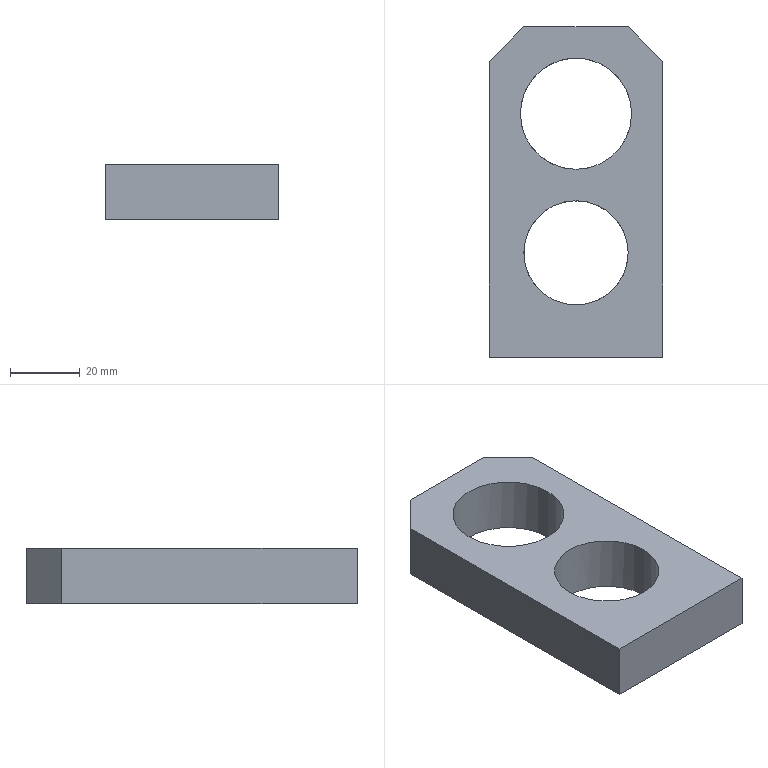Part | NX | features DATUM_CSYS 1, EXTRACT_DATUM_PLANE 1, EXTRUDE 1, SKETCH 1 | 1 solid | 10 faces | box 50 x 95 x 16 mm | volume 50222 mm3 | plane 8 | cylinder 2 | commonest cylinder face diameters 30 x1 32 x1
STEP:
#1=CARTESIAN_POINT('',(-25.,15.,16.));
#2=VERTEX_POINT('',#1);
#3=CARTESIAN_POINT('',(-25.,-70.,16.));
#4=VERTEX_POINT('',#3);
#5=CARTESIAN_POINT('',(-25.,15.,16.));
#6=DIRECTION('',(0.,-1.,0.));
#7=VECTOR('',#6,1000.);
#8=LINE('',#5,#7);
#9=EDGE_CURVE('',#2,#4,#8,.T.);
#10=ORIENTED_EDGE('',*,*,#9,.F.);
#11=CARTESIAN_POINT('',(-25.,15.,0.));
#12=VERTEX_POINT('',#11);
#13=CARTESIAN_POINT('',(-25.,15.,0.));
#14=DIRECTION('',(0.,0.,1.));
#15=VECTOR('',#14,1000.);
#16=LINE('',#13,#15);
#17=EDGE_CURVE('',#12,#2,#16,.T.);
#18=ORIENTED_EDGE('',*,*,#17,.F.);
#19=CARTESIAN_POINT('',(-25.,-70.,0.));
#20=VERTEX_POINT('',#19);
#21=CARTESIAN_POINT('',(-25.,15.,0.));
#22=DIRECTION('',(0.,-1.,0.));
#23=VECTOR('',#22,1000.);
#24=LINE('',#21,#23);
#25=EDGE_CURVE('',#12,#20,#24,.T.);
#26=ORIENTED_EDGE('',*,*,#25,.T.);
#27=CARTESIAN_POINT('',(-25.,-70.,0.));
#28=DIRECTION('',(0.,0.,1.));
#29=VECTOR('',#28,1000.);
#30=LINE('',#27,#29);
#31=EDGE_CURVE('',#20,#4,#30,.T.);
#32=ORIENTED_EDGE('',*,*,#31,.T.);
#33=EDGE_LOOP('',(#10,#18,#26,#32));
#34=FACE_BOUND('',#33,.T.);
#35=CARTESIAN_POINT('',(-25.,15.,0.));
#36=DIRECTION('',(-1.,0.,0.));
#37=DIRECTION('',(0.,0.,1.));
#38=AXIS2_PLACEMENT_3D('',#35,#36,#37);
#39=PLANE('',#38);
#40=ADVANCED_FACE('',(#34),#39,.T.);
#41=CARTESIAN_POINT('',(25.,-70.,16.));
#42=VERTEX_POINT('',#41);
#43=CARTESIAN_POINT('',(-25.,-70.,16.));
#44=DIRECTION('',(1.,0.,0.));
#45=VECTOR('',#44,1000.);
#46=LINE('',#43,#45);
#47=EDGE_CURVE('',#4,#42,#46,.T.);
#48=ORIENTED_EDGE('',*,*,#47,.F.);
#49=ORIENTED_EDGE('',*,*,#31,.F.);
#50=CARTESIAN_POINT('',(25.,-70.,0.));
#51=VERTEX_POINT('',#50);
#52=CARTESIAN_POINT('',(-25.,-70.,0.));
#53=DIRECTION('',(1.,0.,0.));
#54=VECTOR('',#53,1000.);
#55=LINE('',#52,#54);
#56=EDGE_CURVE('',#20,#51,#55,.T.);
#57=ORIENTED_EDGE('',*,*,#56,.T.);
#58=CARTESIAN_POINT('',(25.,-70.,0.));
#59=DIRECTION('',(0.,0.,1.));
#60=VECTOR('',#59,1000.);
#61=LINE('',#58,#60);
#62=EDGE_CURVE('',#51,#42,#61,.T.);
#63=ORIENTED_EDGE('',*,*,#62,.T.);
#64=EDGE_LOOP('',(#48,#49,#57,#63));
#65=FACE_BOUND('',#64,.T.);
#66=CARTESIAN_POINT('',(-25.,-70.,0.));
#67=DIRECTION('',(0.,-1.,0.));
#68=DIRECTION('',(0.,0.,-1.));
#69=AXIS2_PLACEMENT_3D('',#66,#67,#68);
#70=PLANE('',#69);
#71=ADVANCED_FACE('',(#65),#70,.T.);
#72=CARTESIAN_POINT('',(25.,15.,16.));
#73=VERTEX_POINT('',#72);
#74=CARTESIAN_POINT('',(25.,-70.,16.));
#75=DIRECTION('',(0.,1.,0.));
#76=VECTOR('',#75,1000.);
#77=LINE('',#74,#76);
#78=EDGE_CURVE('',#42,#73,#77,.T.);
#79=ORIENTED_EDGE('',*,*,#78,.F.);
#80=ORIENTED_EDGE('',*,*,#62,.F.);
#81=CARTESIAN_POINT('',(25.,15.,0.));
#82=VERTEX_POINT('',#81);
#83=CARTESIAN_POINT('',(25.,-70.,0.));
#84=DIRECTION('',(0.,1.,0.));
#85=VECTOR('',#84,1000.);
#86=LINE('',#83,#85);
#87=EDGE_CURVE('',#51,#82,#86,.T.);
#88=ORIENTED_EDGE('',*,*,#87,.T.);
#89=CARTESIAN_POINT('',(25.,15.,0.));
#90=DIRECTION('',(0.,0.,1.));
#91=VECTOR('',#90,1000.);
#92=LINE('',#89,#91);
#93=EDGE_CURVE('',#82,#73,#92,.T.);
#94=ORIENTED_EDGE('',*,*,#93,.T.);
#95=EDGE_LOOP('',(#79,#80,#88,#94));
#96=FACE_BOUND('',#95,.T.);
#97=CARTESIAN_POINT('',(25.,-70.,0.));
#98=DIRECTION('',(1.,0.,0.));
#99=DIRECTION('',(0.,0.,-1.));
#100=AXIS2_PLACEMENT_3D('',#97,#98,#99);
#101=PLANE('',#100);
#102=ADVANCED_FACE('',(#96),#101,.T.);
#103=CARTESIAN_POINT('',(15.,25.,16.));
#104=VERTEX_POINT('',#103);
#105=CARTESIAN_POINT('',(25.,15.,16.));
#106=DIRECTION('',(-0.7071,0.7071,0.));
#107=VECTOR('',#106,1000.);
#108=LINE('',#105,#107);
#109=EDGE_CURVE('',#73,#104,#108,.T.);
#110=ORIENTED_EDGE('',*,*,#109,.F.);
#111=ORIENTED_EDGE('',*,*,#93,.F.);
#112=CARTESIAN_POINT('',(15.,25.,0.));
#113=VERTEX_POINT('',#112);
#114=CARTESIAN_POINT('',(25.,15.,0.));
#115=DIRECTION('',(-0.7071,0.7071,0.));
#116=VECTOR('',#115,1000.);
#117=LINE('',#114,#116);
#118=EDGE_CURVE('',#82,#113,#117,.T.);
#119=ORIENTED_EDGE('',*,*,#118,.T.);
#120=CARTESIAN_POINT('',(15.,25.,0.));
#121=DIRECTION('',(0.,0.,1.));
#122=VECTOR('',#121,1000.);
#123=LINE('',#120,#122);
#124=EDGE_CURVE('',#113,#104,#123,.T.);
#125=ORIENTED_EDGE('',*,*,#124,.T.);
#126=EDGE_LOOP('',(#110,#111,#119,#125));
#127=FACE_BOUND('',#126,.T.);
#128=CARTESIAN_POINT('',(25.,15.,0.));
#129=DIRECTION('',(0.7071,0.7071,0.));
#130=DIRECTION('',(-0.7071,0.7071,0.));
#131=AXIS2_PLACEMENT_3D('',#128,#129,#130);
#132=PLANE('',#131);
#133=ADVANCED_FACE('',(#127),#132,.T.);
#134=CARTESIAN_POINT('',(-15.,25.,16.));
#135=VERTEX_POINT('',#134);
#136=CARTESIAN_POINT('',(15.,25.,16.));
#137=DIRECTION('',(-1.,0.,0.));
#138=VECTOR('',#137,1000.);
#139=LINE('',#136,#138);
#140=EDGE_CURVE('',#104,#135,#139,.T.);
#141=ORIENTED_EDGE('',*,*,#140,.F.);
#142=ORIENTED_EDGE('',*,*,#124,.F.);
#143=CARTESIAN_POINT('',(-15.,25.,0.));
#144=VERTEX_POINT('',#143);
#145=CARTESIAN_POINT('',(15.,25.,0.));
#146=DIRECTION('',(-1.,0.,0.));
#147=VECTOR('',#146,1000.);
#148=LINE('',#145,#147);
#149=EDGE_CURVE('',#113,#144,#148,.T.);
#150=ORIENTED_EDGE('',*,*,#149,.T.);
#151=CARTESIAN_POINT('',(-15.,25.,0.));
#152=DIRECTION('',(0.,0.,1.));
#153=VECTOR('',#152,1000.);
#154=LINE('',#151,#153);
#155=EDGE_CURVE('',#144,#135,#154,.T.);
#156=ORIENTED_EDGE('',*,*,#155,.T.);
#157=EDGE_LOOP('',(#141,#142,#150,#156));
#158=FACE_BOUND('',#157,.T.);
#159=CARTESIAN_POINT('',(15.,25.,0.));
#160=DIRECTION('',(0.,1.,0.));
#161=DIRECTION('',(0.,0.,1.));
#162=AXIS2_PLACEMENT_3D('',#159,#160,#161);
#163=PLANE('',#162);
#164=ADVANCED_FACE('',(#158),#163,.T.);
#165=CARTESIAN_POINT('',(-16.,0.,16.));
#166=VERTEX_POINT('',#165);
#167=CARTESIAN_POINT('',(0.,0.,16.));
#168=DIRECTION('',(0.,0.,-1.));
#169=DIRECTION('',(-1.,0.,0.));
#170=AXIS2_PLACEMENT_3D('',#167,#168,#169);
#171=CIRCLE('',#170,16.);
#172=EDGE_CURVE('',#166,#166,#171,.T.);
#173=ORIENTED_EDGE('',*,*,#172,.F.);
#174=EDGE_LOOP('',(#173));
#175=FACE_BOUND('',#174,.T.);
#176=CARTESIAN_POINT('',(16.,0.,0.));
#177=VERTEX_POINT('',#176);
#178=CARTESIAN_POINT('',(0.,0.,0.));
#179=DIRECTION('',(0.,0.,-1.));
#180=DIRECTION('',(1.,0.,0.));
#181=AXIS2_PLACEMENT_3D('',#178,#179,#180);
#182=CIRCLE('',#181,16.);
#183=EDGE_CURVE('',#177,#177,#182,.T.);
#184=ORIENTED_EDGE('',*,*,#183,.T.);
#185=EDGE_LOOP('',(#184));
#186=FACE_BOUND('',#185,.T.);
#187=CARTESIAN_POINT('',(0.,0.,0.));
#188=DIRECTION('',(0.,0.,1.));
#189=DIRECTION('',(1.,0.,0.));
#190=AXIS2_PLACEMENT_3D('',#187,#188,#189);
#191=CYLINDRICAL_SURFACE('',#190,16.);
#192=ADVANCED_FACE('',(#175,#186),#191,.F.);
#193=CARTESIAN_POINT('',(-15.,25.,16.));
#194=DIRECTION('',(-0.7071,-0.7071,0.));
#195=VECTOR('',#194,1000.);
#196=LINE('',#193,#195);
#197=EDGE_CURVE('',#135,#2,#196,.T.);
#198=ORIENTED_EDGE('',*,*,#197,.F.);
#199=ORIENTED_EDGE('',*,*,#155,.F.);
#200=CARTESIAN_POINT('',(-15.,25.,0.));
#201=DIRECTION('',(-0.7071,-0.7071,0.));
#202=VECTOR('',#201,1000.);
#203=LINE('',#200,#202);
#204=EDGE_CURVE('',#144,#12,#203,.T.);
#205=ORIENTED_EDGE('',*,*,#204,.T.);
#206=ORIENTED_EDGE('',*,*,#17,.T.);
#207=EDGE_LOOP('',(#198,#199,#205,#206));
#208=FACE_BOUND('',#207,.T.);
#209=CARTESIAN_POINT('',(-15.,25.,0.));
#210=DIRECTION('',(-0.7071,0.7071,0.));
#211=DIRECTION('',(-0.7071,-0.7071,0.));
#212=AXIS2_PLACEMENT_3D('',#209,#210,#211);
#213=PLANE('',#212);
#214=ADVANCED_FACE('',(#208),#213,.T.);
#215=CARTESIAN_POINT('',(-15.,-40.,16.));
#216=VERTEX_POINT('',#215);
#217=CARTESIAN_POINT('',(0.,-40.,16.));
#218=DIRECTION('',(0.,0.,-1.));
#219=DIRECTION('',(-1.,0.,0.));
#220=AXIS2_PLACEMENT_3D('',#217,#218,#219);
#221=CIRCLE('',#220,15.);
#222=EDGE_CURVE('',#216,#216,#221,.T.);
#223=ORIENTED_EDGE('',*,*,#222,.F.);
#224=EDGE_LOOP('',(#223));
#225=FACE_BOUND('',#224,.T.);
#226=CARTESIAN_POINT('',(15.,-40.,0.));
#227=VERTEX_POINT('',#226);
#228=CARTESIAN_POINT('',(0.,-40.,0.));
#229=DIRECTION('',(0.,0.,-1.));
#230=DIRECTION('',(1.,0.,0.));
#231=AXIS2_PLACEMENT_3D('',#228,#229,#230);
#232=CIRCLE('',#231,15.);
#233=EDGE_CURVE('',#227,#227,#232,.T.);
#234=ORIENTED_EDGE('',*,*,#233,.T.);
#235=EDGE_LOOP('',(#234));
#236=FACE_BOUND('',#235,.T.);
#237=CARTESIAN_POINT('',(0.,-40.,0.));
#238=DIRECTION('',(0.,0.,1.));
#239=DIRECTION('',(1.,0.,0.));
#240=AXIS2_PLACEMENT_3D('',#237,#238,#239);
#241=CYLINDRICAL_SURFACE('',#240,15.);
#242=ADVANCED_FACE('',(#225,#236),#241,.F.);
#243=ORIENTED_EDGE('',*,*,#25,.F.);
#244=ORIENTED_EDGE('',*,*,#204,.F.);
#245=ORIENTED_EDGE('',*,*,#149,.F.);
#246=ORIENTED_EDGE('',*,*,#118,.F.);
#247=ORIENTED_EDGE('',*,*,#87,.F.);
#248=ORIENTED_EDGE('',*,*,#56,.F.);
#249=EDGE_LOOP('',(#243,#244,#245,#246,#247,#248));
#250=FACE_BOUND('',#249,.T.);
#251=ORIENTED_EDGE('',*,*,#183,.F.);
#252=EDGE_LOOP('',(#251));
#253=FACE_BOUND('',#252,.T.);
#254=ORIENTED_EDGE('',*,*,#233,.F.);
#255=EDGE_LOOP('',(#254));
#256=FACE_BOUND('',#255,.T.);
#257=CARTESIAN_POINT('',(0.,0.,0.));
#258=DIRECTION('',(0.,0.,-1.));
#259=DIRECTION('',(-1.,0.,0.));
#260=AXIS2_PLACEMENT_3D('',#257,#258,#259);
#261=PLANE('',#260);
#262=ADVANCED_FACE('',(#250,#253,#256),#261,.T.);
#263=ORIENTED_EDGE('',*,*,#9,.T.);
#264=ORIENTED_EDGE('',*,*,#47,.T.);
#265=ORIENTED_EDGE('',*,*,#78,.T.);
#266=ORIENTED_EDGE('',*,*,#109,.T.);
#267=ORIENTED_EDGE('',*,*,#140,.T.);
#268=ORIENTED_EDGE('',*,*,#197,.T.);
#269=EDGE_LOOP('',(#263,#264,#265,#266,#267,#268));
#270=FACE_BOUND('',#269,.T.);
#271=ORIENTED_EDGE('',*,*,#172,.T.);
#272=EDGE_LOOP('',(#271));
#273=FACE_BOUND('',#272,.T.);
#274=ORIENTED_EDGE('',*,*,#222,.T.);
#275=EDGE_LOOP('',(#274));
#276=FACE_BOUND('',#275,.T.);
#277=CARTESIAN_POINT('',(0.,0.,16.));
#278=DIRECTION('',(0.,0.,-1.));
#279=DIRECTION('',(-1.,0.,0.));
#280=AXIS2_PLACEMENT_3D('',#277,#278,#279);
#281=PLANE('',#280);
#282=ADVANCED_FACE('',(#270,#273,#276),#281,.F.);
#283=CLOSED_SHELL('',(#40,#71,#102,#133,#164,#192,#214,#242,#262,#282));
#284=MANIFOLD_SOLID_BREP('',#283);
#285=(LENGTH_UNIT()NAMED_UNIT(*)SI_UNIT(.MILLI.,.METRE.));
#286=UNCERTAINTY_MEASURE_WITH_UNIT(LENGTH_MEASURE(0.00001),#285,'','');
#287=(NAMED_UNIT(*)PLANE_ANGLE_UNIT()SI_UNIT($,.RADIAN.));
#288=(NAMED_UNIT(*)SI_UNIT($,.STERADIAN.)SOLID_ANGLE_UNIT());
#289=(GEOMETRIC_REPRESENTATION_CONTEXT(3)GLOBAL_UNCERTAINTY_ASSIGNED_CONTEXT((#286))GLOBAL_UNIT_ASSIGNED_CONTEXT((#285,#287,#288))REPRESENTATION_CONTEXT('',''));
#290=ADVANCED_BREP_SHAPE_REPRESENTATION('',(#284),#289);